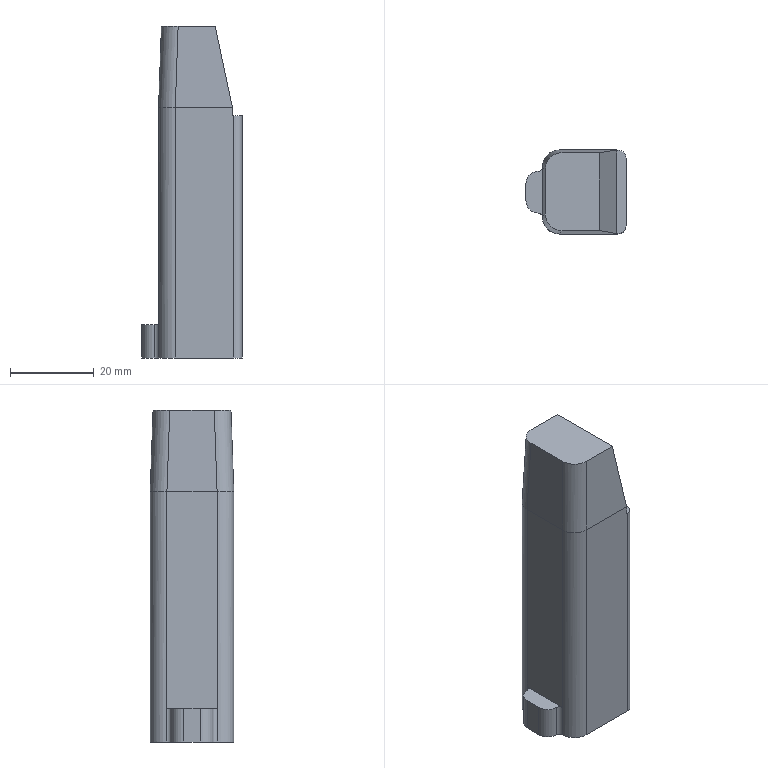Part | STEP file | solid 47 | 1 solid | 24 faces | box 24 x 20 x 79.442 mm | volume 29301 mm3 | plane 14 | cylinder 10 | commonest cylinder face diameters 8 x4 2 x2 4 x2 6 x2